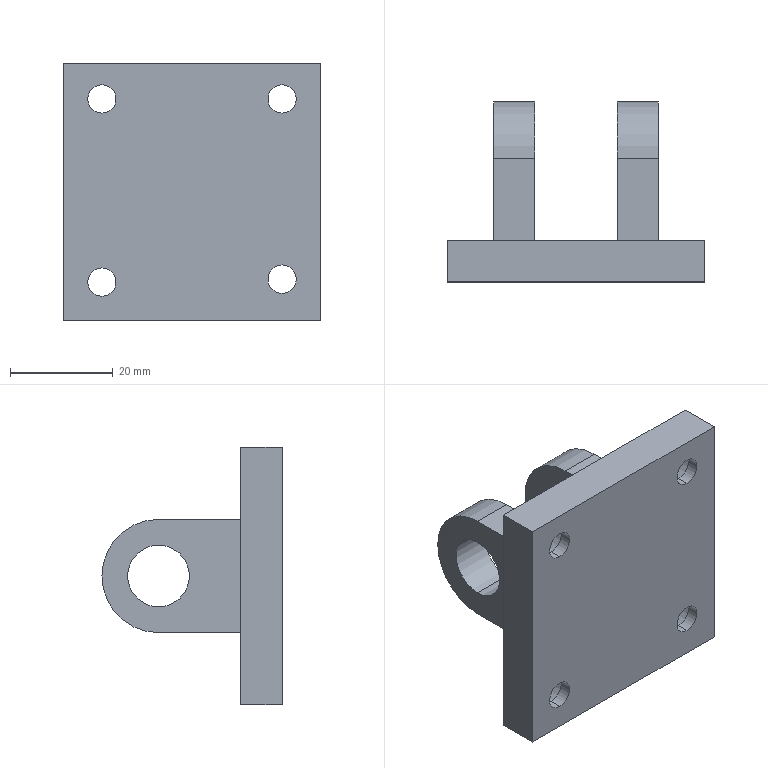Part | STEP file | X77-03301 | 1 solid | 42 faces | box 50 x 35 x 50 mm | volume 24854 mm3 | cylinder 24 | plane 18 | commonest cylinder face diameters 5.5 x8 10 x8 12 x4 22 x4
STEP:
#1=CARTESIAN_POINT('',(-1969.202,2.3,2.5));
#2=VERTEX_POINT('',#1);
#3=CARTESIAN_POINT('',(-1969.202,2.3,12.5));
#4=VERTEX_POINT('',#3);
#5=CARTESIAN_POINT('',(-1969.202,2.3,7.5));
#6=DIRECTION('',(0.,1.,0.));
#7=DIRECTION('',(0.,0.,1.));
#8=AXIS2_PLACEMENT_3D('',#5,#6,#7);
#9=CIRCLE('',#8,5.);
#10=EDGE_CURVE('',#2,#4,#9,.T.);
#11=ORIENTED_EDGE('',*,*,#10,.F.);
#12=CARTESIAN_POINT('',(-1969.202,8.,2.5));
#13=VERTEX_POINT('',#12);
#14=CARTESIAN_POINT('',(-1969.202,8.,2.5));
#15=DIRECTION('',(0.,1.,0.));
#16=VECTOR('',#15,1000.);
#17=LINE('',#14,#16);
#18=EDGE_CURVE('',#2,#13,#17,.T.);
#19=ORIENTED_EDGE('',*,*,#18,.T.);
#20=CARTESIAN_POINT('',(-1969.202,8.,12.5));
#21=VERTEX_POINT('',#20);
#22=CARTESIAN_POINT('',(-1969.202,8.,7.5));
#23=DIRECTION('',(0.,1.,0.));
#24=DIRECTION('',(0.,0.,1.));
#25=AXIS2_PLACEMENT_3D('',#22,#23,#24);
#26=CIRCLE('',#25,5.);
#27=EDGE_CURVE('',#13,#21,#26,.T.);
#28=ORIENTED_EDGE('',*,*,#27,.T.);
#29=CARTESIAN_POINT('',(-1969.202,8.,12.5));
#30=DIRECTION('',(0.,1.,0.));
#31=VECTOR('',#30,1000.);
#32=LINE('',#29,#31);
#33=EDGE_CURVE('',#4,#21,#32,.T.);
#34=ORIENTED_EDGE('',*,*,#33,.F.);
#35=EDGE_LOOP('',(#11,#19,#28,#34));
#36=FACE_OUTER_BOUND('',#35,.T.);
#37=CARTESIAN_POINT('',(-1969.202,8.,7.5));
#38=DIRECTION('',(0.,1.,0.));
#39=DIRECTION('',(0.,0.,1.));
#40=AXIS2_PLACEMENT_3D('',#37,#38,#39);
#41=CYLINDRICAL_SURFACE('',#40,5.);
#42=ADVANCED_FACE('',(#36),#41,.F.);
#43=CARTESIAN_POINT('',(-1969.202,0.,4.75));
#44=VERTEX_POINT('',#43);
#45=CARTESIAN_POINT('',(-1969.202,0.,10.25));
#46=VERTEX_POINT('',#45);
#47=CARTESIAN_POINT('',(-1969.202,0.,7.5));
#48=DIRECTION('',(0.,1.,0.));
#49=DIRECTION('',(0.,0.,1.));
#50=AXIS2_PLACEMENT_3D('',#47,#48,#49);
#51=CIRCLE('',#50,2.75);
#52=EDGE_CURVE('',#44,#46,#51,.T.);
#53=ORIENTED_EDGE('',*,*,#52,.F.);
#54=CARTESIAN_POINT('',(-1969.202,2.3,4.75));
#55=VERTEX_POINT('',#54);
#56=CARTESIAN_POINT('',(-1969.202,8.,4.75));
#57=DIRECTION('',(0.,1.,0.));
#58=VECTOR('',#57,1000.);
#59=LINE('',#56,#58);
#60=EDGE_CURVE('',#44,#55,#59,.T.);
#61=ORIENTED_EDGE('',*,*,#60,.T.);
#62=CARTESIAN_POINT('',(-1969.202,2.3,10.25));
#63=VERTEX_POINT('',#62);
#64=CARTESIAN_POINT('',(-1969.202,2.3,7.5));
#65=DIRECTION('',(0.,1.,0.));
#66=DIRECTION('',(0.,0.,1.));
#67=AXIS2_PLACEMENT_3D('',#64,#65,#66);
#68=CIRCLE('',#67,2.75);
#69=EDGE_CURVE('',#55,#63,#68,.T.);
#70=ORIENTED_EDGE('',*,*,#69,.T.);
#71=CARTESIAN_POINT('',(-1969.202,8.,10.25));
#72=DIRECTION('',(0.,1.,0.));
#73=VECTOR('',#72,1000.);
#74=LINE('',#71,#73);
#75=EDGE_CURVE('',#46,#63,#74,.T.);
#76=ORIENTED_EDGE('',*,*,#75,.F.);
#77=EDGE_LOOP('',(#53,#61,#70,#76));
#78=FACE_OUTER_BOUND('',#77,.T.);
#79=CARTESIAN_POINT('',(-1969.202,8.,7.5));
#80=DIRECTION('',(0.,1.,0.));
#81=DIRECTION('',(0.,0.,1.));
#82=AXIS2_PLACEMENT_3D('',#79,#80,#81);
#83=CYLINDRICAL_SURFACE('',#82,2.75);
#84=ADVANCED_FACE('',(#78),#83,.F.);
#85=CARTESIAN_POINT('',(-1934.202,2.3,3.072));
#86=VERTEX_POINT('',#85);
#87=CARTESIAN_POINT('',(-1934.202,2.3,13.072));
#88=VERTEX_POINT('',#87);
#89=CARTESIAN_POINT('',(-1934.202,2.3,8.072));
#90=DIRECTION('',(0.,1.,0.));
#91=DIRECTION('',(0.,0.,1.));
#92=AXIS2_PLACEMENT_3D('',#89,#90,#91);
#93=CIRCLE('',#92,5.);
#94=EDGE_CURVE('',#86,#88,#93,.T.);
#95=ORIENTED_EDGE('',*,*,#94,.F.);
#96=CARTESIAN_POINT('',(-1934.202,8.,3.072));
#97=VERTEX_POINT('',#96);
#98=CARTESIAN_POINT('',(-1934.202,8.,3.072));
#99=DIRECTION('',(0.,1.,0.));
#100=VECTOR('',#99,1000.);
#101=LINE('',#98,#100);
#102=EDGE_CURVE('',#86,#97,#101,.T.);
#103=ORIENTED_EDGE('',*,*,#102,.T.);
#104=CARTESIAN_POINT('',(-1934.202,8.,13.072));
#105=VERTEX_POINT('',#104);
#106=CARTESIAN_POINT('',(-1934.202,8.,8.072));
#107=DIRECTION('',(0.,1.,0.));
#108=DIRECTION('',(0.,0.,1.));
#109=AXIS2_PLACEMENT_3D('',#106,#107,#108);
#110=CIRCLE('',#109,5.);
#111=EDGE_CURVE('',#97,#105,#110,.T.);
#112=ORIENTED_EDGE('',*,*,#111,.T.);
#113=CARTESIAN_POINT('',(-1934.202,8.,13.072));
#114=DIRECTION('',(0.,1.,0.));
#115=VECTOR('',#114,1000.);
#116=LINE('',#113,#115);
#117=EDGE_CURVE('',#88,#105,#116,.T.);
#118=ORIENTED_EDGE('',*,*,#117,.F.);
#119=EDGE_LOOP('',(#95,#103,#112,#118));
#120=FACE_OUTER_BOUND('',#119,.T.);
#121=CARTESIAN_POINT('',(-1934.202,8.,8.072));
#122=DIRECTION('',(0.,1.,0.));
#123=DIRECTION('',(0.,0.,1.));
#124=AXIS2_PLACEMENT_3D('',#121,#122,#123);
#125=CYLINDRICAL_SURFACE('',#124,5.);
#126=ADVANCED_FACE('',(#120),#125,.F.);
#127=CARTESIAN_POINT('',(-1934.202,0.,5.322));
#128=VERTEX_POINT('',#127);
#129=CARTESIAN_POINT('',(-1934.202,0.,10.822));
#130=VERTEX_POINT('',#129);
#131=CARTESIAN_POINT('',(-1934.202,0.,8.072));
#132=DIRECTION('',(0.,1.,0.));
#133=DIRECTION('',(0.,0.,1.));
#134=AXIS2_PLACEMENT_3D('',#131,#132,#133);
#135=CIRCLE('',#134,2.75);
#136=EDGE_CURVE('',#128,#130,#135,.T.);
#137=ORIENTED_EDGE('',*,*,#136,.F.);
#138=CARTESIAN_POINT('',(-1934.202,2.3,5.322));
#139=VERTEX_POINT('',#138);
#140=CARTESIAN_POINT('',(-1934.202,8.,5.322));
#141=DIRECTION('',(0.,1.,0.));
#142=VECTOR('',#141,1000.);
#143=LINE('',#140,#142);
#144=EDGE_CURVE('',#128,#139,#143,.T.);
#145=ORIENTED_EDGE('',*,*,#144,.T.);
#146=CARTESIAN_POINT('',(-1934.202,2.3,10.822));
#147=VERTEX_POINT('',#146);
#148=CARTESIAN_POINT('',(-1934.202,2.3,8.072));
#149=DIRECTION('',(0.,1.,0.));
#150=DIRECTION('',(0.,0.,1.));
#151=AXIS2_PLACEMENT_3D('',#148,#149,#150);
#152=CIRCLE('',#151,2.75);
#153=EDGE_CURVE('',#139,#147,#152,.T.);
#154=ORIENTED_EDGE('',*,*,#153,.T.);
#155=CARTESIAN_POINT('',(-1934.202,8.,10.822));
#156=DIRECTION('',(0.,1.,0.));
#157=VECTOR('',#156,1000.);
#158=LINE('',#155,#157);
#159=EDGE_CURVE('',#130,#147,#158,.T.);
#160=ORIENTED_EDGE('',*,*,#159,.F.);
#161=EDGE_LOOP('',(#137,#145,#154,#160));
#162=FACE_OUTER_BOUND('',#161,.T.);
#163=CARTESIAN_POINT('',(-1934.202,8.,8.072));
#164=DIRECTION('',(0.,1.,0.));
#165=DIRECTION('',(0.,0.,1.));
#166=AXIS2_PLACEMENT_3D('',#163,#164,#165);
#167=CYLINDRICAL_SURFACE('',#166,2.75);
#168=ADVANCED_FACE('',(#162),#167,.F.);
#169=CARTESIAN_POINT('',(-1934.202,2.3,38.072));
#170=VERTEX_POINT('',#169);
#171=CARTESIAN_POINT('',(-1934.202,2.3,48.072));
#172=VERTEX_POINT('',#171);
#173=CARTESIAN_POINT('',(-1934.202,2.3,43.072));
#174=DIRECTION('',(0.,1.,0.));
#175=DIRECTION('',(0.,0.,1.));
#176=AXIS2_PLACEMENT_3D('',#173,#174,#175);
#177=CIRCLE('',#176,5.);
#178=EDGE_CURVE('',#170,#172,#177,.T.);
#179=ORIENTED_EDGE('',*,*,#178,.F.);
#180=CARTESIAN_POINT('',(-1934.202,8.,38.072));
#181=VERTEX_POINT('',#180);
#182=CARTESIAN_POINT('',(-1934.202,8.,38.072));
#183=DIRECTION('',(0.,1.,0.));
#184=VECTOR('',#183,1000.);
#185=LINE('',#182,#184);
#186=EDGE_CURVE('',#170,#181,#185,.T.);
#187=ORIENTED_EDGE('',*,*,#186,.T.);
#188=CARTESIAN_POINT('',(-1934.202,8.,48.072));
#189=VERTEX_POINT('',#188);
#190=CARTESIAN_POINT('',(-1934.202,8.,43.072));
#191=DIRECTION('',(0.,1.,0.));
#192=DIRECTION('',(0.,0.,1.));
#193=AXIS2_PLACEMENT_3D('',#190,#191,#192);
#194=CIRCLE('',#193,5.);
#195=EDGE_CURVE('',#181,#189,#194,.T.);
#196=ORIENTED_EDGE('',*,*,#195,.T.);
#197=CARTESIAN_POINT('',(-1934.202,8.,48.072));
#198=DIRECTION('',(0.,1.,0.));
#199=VECTOR('',#198,1000.);
#200=LINE('',#197,#199);
#201=EDGE_CURVE('',#172,#189,#200,.T.);
#202=ORIENTED_EDGE('',*,*,#201,.F.);
#203=EDGE_LOOP('',(#179,#187,#196,#202));
#204=FACE_OUTER_BOUND('',#203,.T.);
#205=CARTESIAN_POINT('',(-1934.202,8.,43.072));
#206=DIRECTION('',(0.,1.,0.));
#207=DIRECTION('',(0.,0.,1.));
#208=AXIS2_PLACEMENT_3D('',#205,#206,#207);
#209=CYLINDRICAL_SURFACE('',#208,5.);
#210=ADVANCED_FACE('',(#204),#209,.F.);
#211=CARTESIAN_POINT('',(-1934.202,0.,40.322));
#212=VERTEX_POINT('',#211);
#213=CARTESIAN_POINT('',(-1934.202,0.,45.822));
#214=VERTEX_POINT('',#213);
#215=CARTESIAN_POINT('',(-1934.202,0.,43.072));
#216=DIRECTION('',(0.,1.,0.));
#217=DIRECTION('',(0.,0.,1.));
#218=AXIS2_PLACEMENT_3D('',#215,#216,#217);
#219=CIRCLE('',#218,2.75);
#220=EDGE_CURVE('',#212,#214,#219,.T.);
#221=ORIENTED_EDGE('',*,*,#220,.F.);
#222=CARTESIAN_POINT('',(-1934.202,2.3,40.322));
#223=VERTEX_POINT('',#222);
#224=CARTESIAN_POINT('',(-1934.202,8.,40.322));
#225=DIRECTION('',(0.,1.,0.));
#226=VECTOR('',#225,1000.);
#227=LINE('',#224,#226);
#228=EDGE_CURVE('',#212,#223,#227,.T.);
#229=ORIENTED_EDGE('',*,*,#228,.T.);
#230=CARTESIAN_POINT('',(-1934.202,2.3,45.822));
#231=VERTEX_POINT('',#230);
#232=CARTESIAN_POINT('',(-1934.202,2.3,43.072));
#233=DIRECTION('',(0.,1.,0.));
#234=DIRECTION('',(0.,0.,1.));
#235=AXIS2_PLACEMENT_3D('',#232,#233,#234);
#236=CIRCLE('',#235,2.75);
#237=EDGE_CURVE('',#223,#231,#236,.T.);
#238=ORIENTED_EDGE('',*,*,#237,.T.);
#239=CARTESIAN_POINT('',(-1934.202,8.,45.822));
#240=DIRECTION('',(0.,1.,0.));
#241=VECTOR('',#240,1000.);
#242=LINE('',#239,#241);
#243=EDGE_CURVE('',#214,#231,#242,.T.);
#244=ORIENTED_EDGE('',*,*,#243,.F.);
#245=EDGE_LOOP('',(#221,#229,#238,#244));
#246=FACE_OUTER_BOUND('',#245,.T.);
#247=CARTESIAN_POINT('',(-1934.202,8.,43.072));
#248=DIRECTION('',(0.,1.,0.));
#249=DIRECTION('',(0.,0.,1.));
#250=AXIS2_PLACEMENT_3D('',#247,#248,#249);
#251=CYLINDRICAL_SURFACE('',#250,2.75);
#252=ADVANCED_FACE('',(#246),#251,.F.);
#253=CARTESIAN_POINT('',(-1969.202,2.3,38.072));
#254=VERTEX_POINT('',#253);
#255=CARTESIAN_POINT('',(-1969.202,2.3,48.072));
#256=VERTEX_POINT('',#255);
#257=CARTESIAN_POINT('',(-1969.202,2.3,43.072));
#258=DIRECTION('',(0.,1.,0.));
#259=DIRECTION('',(0.,0.,1.));
#260=AXIS2_PLACEMENT_3D('',#257,#258,#259);
#261=CIRCLE('',#260,5.);
#262=EDGE_CURVE('',#254,#256,#261,.T.);
#263=ORIENTED_EDGE('',*,*,#262,.F.);
#264=CARTESIAN_POINT('',(-1969.202,8.,38.072));
#265=VERTEX_POINT('',#264);
#266=CARTESIAN_POINT('',(-1969.202,8.,38.072));
#267=DIRECTION('',(0.,1.,0.));
#268=VECTOR('',#267,1000.);
#269=LINE('',#266,#268);
#270=EDGE_CURVE('',#254,#265,#269,.T.);
#271=ORIENTED_EDGE('',*,*,#270,.T.);
#272=CARTESIAN_POINT('',(-1969.202,8.,48.072));
#273=VERTEX_POINT('',#272);
#274=CARTESIAN_POINT('',(-1969.202,8.,43.072));
#275=DIRECTION('',(0.,1.,0.));
#276=DIRECTION('',(0.,0.,1.));
#277=AXIS2_PLACEMENT_3D('',#274,#275,#276);
#278=CIRCLE('',#277,5.);
#279=EDGE_CURVE('',#265,#273,#278,.T.);
#280=ORIENTED_EDGE('',*,*,#279,.T.);
#281=CARTESIAN_POINT('',(-1969.202,8.,48.072));
#282=DIRECTION('',(0.,1.,0.));
#283=VECTOR('',#282,1000.);
#284=LINE('',#281,#283);
#285=EDGE_CURVE('',#256,#273,#284,.T.);
#286=ORIENTED_EDGE('',*,*,#285,.F.);
#287=EDGE_LOOP('',(#263,#271,#280,#286));
#288=FACE_OUTER_BOUND('',#287,.T.);
#289=CARTESIAN_POINT('',(-1969.202,8.,43.072));
#290=DIRECTION('',(0.,1.,0.));
#291=DIRECTION('',(0.,0.,1.));
#292=AXIS2_PLACEMENT_3D('',#289,#290,#291);
#293=CYLINDRICAL_SURFACE('',#292,5.);
#294=ADVANCED_FACE('',(#288),#293,.F.);
#295=CARTESIAN_POINT('',(-1969.202,0.,40.322));
#296=VERTEX_POINT('',#295);
#297=CARTESIAN_POINT('',(-1969.202,0.,45.822));
#298=VERTEX_POINT('',#297);
#299=CARTESIAN_POINT('',(-1969.202,0.,43.072));
#300=DIRECTION('',(0.,1.,0.));
#301=DIRECTION('',(0.,0.,1.));
#302=AXIS2_PLACEMENT_3D('',#299,#300,#301);
#303=CIRCLE('',#302,2.75);
#304=EDGE_CURVE('',#296,#298,#303,.T.);
#305=ORIENTED_EDGE('',*,*,#304,.F.);
#306=CARTESIAN_POINT('',(-1969.202,2.3,40.322));
#307=VERTEX_POINT('',#306);
#308=CARTESIAN_POINT('',(-1969.202,8.,40.322));
#309=DIRECTION('',(0.,1.,0.));
#310=VECTOR('',#309,1000.);
#311=LINE('',#308,#310);
#312=EDGE_CURVE('',#296,#307,#311,.T.);
#313=ORIENTED_EDGE('',*,*,#312,.T.);
#314=CARTESIAN_POINT('',(-1969.202,2.3,45.822));
#315=VERTEX_POINT('',#314);
#316=CARTESIAN_POINT('',(-1969.202,2.3,43.072));
#317=DIRECTION('',(0.,1.,0.));
#318=DIRECTION('',(0.,0.,1.));
#319=AXIS2_PLACEMENT_3D('',#316,#317,#318);
#320=CIRCLE('',#319,2.75);
#321=EDGE_CURVE('',#307,#315,#320,.T.);
#322=ORIENTED_EDGE('',*,*,#321,.T.);
#323=CARTESIAN_POINT('',(-1969.202,8.,45.822));
#324=DIRECTION('',(0.,1.,0.));
#325=VECTOR('',#324,1000.);
#326=LINE('',#323,#325);
#327=EDGE_CURVE('',#298,#315,#326,.T.);
#328=ORIENTED_EDGE('',*,*,#327,.F.);
#329=EDGE_LOOP('',(#305,#313,#322,#328));
#330=FACE_OUTER_BOUND('',#329,.T.);
#331=CARTESIAN_POINT('',(-1969.202,8.,43.072));
#332=DIRECTION('',(0.,1.,0.));
#333=DIRECTION('',(0.,0.,1.));
#334=AXIS2_PLACEMENT_3D('',#331,#332,#333);
#335=CYLINDRICAL_SURFACE('',#334,2.75);
#336=ADVANCED_FACE('',(#330),#335,.F.);
#337=CARTESIAN_POINT('',(-1943.702,24.,31.));
#338=VERTEX_POINT('',#337);
#339=CARTESIAN_POINT('',(-1943.702,24.,19.));
#340=VERTEX_POINT('',#339);
#341=CARTESIAN_POINT('',(-1943.702,24.,25.));
#342=DIRECTION('',(1.,0.,0.));
#343=DIRECTION('',(0.,0.,-1.));
#344=AXIS2_PLACEMENT_3D('',#341,#342,#343);
#345=CIRCLE('',#344,6.);
#346=EDGE_CURVE('',#338,#340,#345,.T.);
#347=ORIENTED_EDGE('',*,*,#346,.F.);
#348=CARTESIAN_POINT('',(-1935.702,24.,31.));
#349=VERTEX_POINT('',#348);
#350=CARTESIAN_POINT('',(-1976.702,24.,31.));
#351=DIRECTION('',(1.,0.,0.));
#352=VECTOR('',#351,1000.);
#353=LINE('',#350,#352);
#354=EDGE_CURVE('',#338,#349,#353,.T.);
#355=ORIENTED_EDGE('',*,*,#354,.T.);
#356=CARTESIAN_POINT('',(-1935.702,24.,19.));
#357=VERTEX_POINT('',#356);
#358=CARTESIAN_POINT('',(-1935.702,24.,25.));
#359=DIRECTION('',(1.,0.,0.));
#360=DIRECTION('',(0.,0.,-1.));
#361=AXIS2_PLACEMENT_3D('',#358,#359,#360);
#362=CIRCLE('',#361,6.);
#363=EDGE_CURVE('',#349,#357,#362,.T.);
#364=ORIENTED_EDGE('',*,*,#363,.T.);
#365=CARTESIAN_POINT('',(-1976.702,24.,19.));
#366=DIRECTION('',(1.,0.,0.));
#367=VECTOR('',#366,1000.);
#368=LINE('',#365,#367);
#369=EDGE_CURVE('',#340,#357,#368,.T.);
#370=ORIENTED_EDGE('',*,*,#369,.F.);
#371=EDGE_LOOP('',(#347,#355,#364,#370));
#372=FACE_OUTER_BOUND('',#371,.T.);
#373=CARTESIAN_POINT('',(-1976.702,24.,25.));
#374=DIRECTION('',(1.,0.,0.));
#375=DIRECTION('',(0.,0.,-1.));
#376=AXIS2_PLACEMENT_3D('',#373,#374,#375);
#377=CYLINDRICAL_SURFACE('',#376,6.);
#378=ADVANCED_FACE('',(#372),#377,.F.);
#379=CARTESIAN_POINT('',(-1967.702,24.,31.));
#380=VERTEX_POINT('',#379);
#381=CARTESIAN_POINT('',(-1967.702,24.,19.));
#382=VERTEX_POINT('',#381);
#383=CARTESIAN_POINT('',(-1967.702,24.,25.));
#384=DIRECTION('',(1.,0.,0.));
#385=DIRECTION('',(0.,0.,-1.));
#386=AXIS2_PLACEMENT_3D('',#383,#384,#385);
#387=CIRCLE('',#386,6.);
#388=EDGE_CURVE('',#380,#382,#387,.T.);
#389=ORIENTED_EDGE('',*,*,#388,.F.);
#390=CARTESIAN_POINT('',(-1959.702,24.,31.));
#391=VERTEX_POINT('',#390);
#392=CARTESIAN_POINT('',(-1976.702,24.,31.));
#393=DIRECTION('',(1.,0.,0.));
#394=VECTOR('',#393,1000.);
#395=LINE('',#392,#394);
#396=EDGE_CURVE('',#380,#391,#395,.T.);
#397=ORIENTED_EDGE('',*,*,#396,.T.);
#398=CARTESIAN_POINT('',(-1959.702,24.,19.));
#399=VERTEX_POINT('',#398);
#400=CARTESIAN_POINT('',(-1959.702,24.,25.));
#401=DIRECTION('',(-1.,0.,0.));
#402=DIRECTION('',(0.,0.,1.));
#403=AXIS2_PLACEMENT_3D('',#400,#401,#402);
#404=CIRCLE('',#403,6.);
#405=EDGE_CURVE('',#399,#391,#404,.T.);
#406=ORIENTED_EDGE('',*,*,#405,.F.);
#407=CARTESIAN_POINT('',(-1976.702,24.,19.));
#408=DIRECTION('',(1.,0.,0.));
#409=VECTOR('',#408,1000.);
#410=LINE('',#407,#409);
#411=EDGE_CURVE('',#382,#399,#410,.T.);
#412=ORIENTED_EDGE('',*,*,#411,.F.);
#413=EDGE_LOOP('',(#389,#397,#406,#412));
#414=FACE_OUTER_BOUND('',#413,.T.);
#415=CARTESIAN_POINT('',(-1976.702,24.,25.));
#416=DIRECTION('',(1.,0.,0.));
#417=DIRECTION('',(0.,0.,-1.));
#418=AXIS2_PLACEMENT_3D('',#415,#416,#417);
#419=CYLINDRICAL_SURFACE('',#418,6.);
#420=ADVANCED_FACE('',(#414),#419,.F.);
#421=CARTESIAN_POINT('',(-1967.702,24.,25.));
#422=DIRECTION('',(1.,0.,0.));
#423=DIRECTION('',(0.,0.,-1.));
#424=AXIS2_PLACEMENT_3D('',#421,#422,#423);
#425=CIRCLE('',#424,6.);
#426=EDGE_CURVE('',#382,#380,#425,.T.);
#427=ORIENTED_EDGE('',*,*,#426,.T.);
#428=ORIENTED_EDGE('',*,*,#388,.T.);
#429=EDGE_LOOP('',(#427,#428));
#430=FACE_BOUND('',#429,.T.);
#431=CARTESIAN_POINT('',(-1967.702,24.,36.));
#432=VERTEX_POINT('',#431);
#433=CARTESIAN_POINT('',(-1967.702,35.,25.));
#434=VERTEX_POINT('',#433);
#435=CARTESIAN_POINT('',(-1967.702,24.,25.));
#436=DIRECTION('',(-1.,0.,0.));
#437=DIRECTION('',(0.,0.,-1.));
#438=AXIS2_PLACEMENT_3D('',#435,#436,#437);
#439=CIRCLE('',#438,11.);
#440=EDGE_CURVE('',#432,#434,#439,.T.);
#441=ORIENTED_EDGE('',*,*,#440,.T.);
#442=CARTESIAN_POINT('',(-1967.702,24.,14.));
#443=VERTEX_POINT('',#442);
#444=CARTESIAN_POINT('',(-1967.702,24.,25.));
#445=DIRECTION('',(-1.,0.,0.));
#446=DIRECTION('',(0.,0.,-1.));
#447=AXIS2_PLACEMENT_3D('',#444,#445,#446);
#448=CIRCLE('',#447,11.);
#449=EDGE_CURVE('',#434,#443,#448,.T.);
#450=ORIENTED_EDGE('',*,*,#449,.T.);
#451=CARTESIAN_POINT('',(-1967.702,8.,14.));
#452=VERTEX_POINT('',#451);
#453=CARTESIAN_POINT('',(-1967.702,8.,14.));
#454=DIRECTION('',(0.,1.,0.));
#455=VECTOR('',#454,1000.);
#456=LINE('',#453,#455);
#457=EDGE_CURVE('',#452,#443,#456,.T.);
#458=ORIENTED_EDGE('',*,*,#457,.F.);
#459=CARTESIAN_POINT('',(-1967.702,8.,36.));
#460=VERTEX_POINT('',#459);
#461=CARTESIAN_POINT('',(-1967.702,8.,50.));
#462=DIRECTION('',(0.,0.,-1.));
#463=VECTOR('',#462,1000.);
#464=LINE('',#461,#463);
#465=EDGE_CURVE('',#460,#452,#464,.T.);
#466=ORIENTED_EDGE('',*,*,#465,.F.);
#467=CARTESIAN_POINT('',(-1967.702,8.,36.));
#468=DIRECTION('',(0.,-1.,0.));
#469=VECTOR('',#468,1000.);
#470=LINE('',#467,#469);
#471=EDGE_CURVE('',#432,#460,#470,.T.);
#472=ORIENTED_EDGE('',*,*,#471,.F.);
#473=EDGE_LOOP('',(#441,#450,#458,#466,#472));
#474=FACE_OUTER_BOUND('',#473,.T.);
#475=CARTESIAN_POINT('',(-1967.702,8.,50.));
#476=DIRECTION('',(1.,0.,0.));
#477=DIRECTION('',(0.,0.,-1.));
#478=AXIS2_PLACEMENT_3D('',#475,#476,#477);
#479=PLANE('',#478);
#480=ADVANCED_FACE('',(#430,#474),#479,.F.);
#481=CARTESIAN_POINT('',(-1935.702,24.,25.));
#482=DIRECTION('',(1.,0.,0.));
#483=DIRECTION('',(0.,0.,-1.));
#484=AXIS2_PLACEMENT_3D('',#481,#482,#483);
#485=CIRCLE('',#484,6.);
#486=EDGE_CURVE('',#357,#349,#485,.T.);
#487=ORIENTED_EDGE('',*,*,#486,.F.);
#488=ORIENTED_EDGE('',*,*,#363,.F.);
#489=EDGE_LOOP('',(#487,#488));
#490=FACE_BOUND('',#489,.T.);
#491=CARTESIAN_POINT('',(-1935.702,8.,14.));
#492=VERTEX_POINT('',#491);
#493=CARTESIAN_POINT('',(-1935.702,24.,14.));
#494=VERTEX_POINT('',#493);
#495=CARTESIAN_POINT('',(-1935.702,21.5,14.));
#496=DIRECTION('',(0.,1.,0.));
#497=VECTOR('',#496,1000.);
#498=LINE('',#495,#497);
#499=EDGE_CURVE('',#492,#494,#498,.T.);
#500=ORIENTED_EDGE('',*,*,#499,.T.);
#501=CARTESIAN_POINT('',(-1935.702,35.,25.));
#502=VERTEX_POINT('',#501);
#503=CARTESIAN_POINT('',(-1935.702,24.,25.));
#504=DIRECTION('',(1.,0.,0.));
#505=DIRECTION('',(0.,0.,1.));
#506=AXIS2_PLACEMENT_3D('',#503,#504,#505);
#507=CIRCLE('',#506,11.);
#508=EDGE_CURVE('',#494,#502,#507,.T.);
#509=ORIENTED_EDGE('',*,*,#508,.T.);
#510=CARTESIAN_POINT('',(-1935.702,24.,36.));
#511=VERTEX_POINT('',#510);
#512=CARTESIAN_POINT('',(-1935.702,24.,25.));
#513=DIRECTION('',(1.,0.,0.));
#514=DIRECTION('',(0.,0.,1.));
#515=AXIS2_PLACEMENT_3D('',#512,#513,#514);
#516=CIRCLE('',#515,11.);
#517=EDGE_CURVE('',#502,#511,#516,.T.);
#518=ORIENTED_EDGE('',*,*,#517,.T.);
#519=CARTESIAN_POINT('',(-1935.702,8.,36.));
#520=VERTEX_POINT('',#519);
#521=CARTESIAN_POINT('',(-1935.702,21.5,36.));
#522=DIRECTION('',(0.,-1.,0.));
#523=VECTOR('',#522,1000.);
#524=LINE('',#521,#523);
#525=EDGE_CURVE('',#511,#520,#524,.T.);
#526=ORIENTED_EDGE('',*,*,#525,.T.);
#527=CARTESIAN_POINT('',(-1935.702,8.,50.));
#528=DIRECTION('',(0.,0.,-1.));
#529=VECTOR('',#528,1000.);
#530=LINE('',#527,#529);
#531=EDGE_CURVE('',#520,#492,#530,.T.);
#532=ORIENTED_EDGE('',*,*,#531,.T.);
#533=EDGE_LOOP('',(#500,#509,#518,#526,#532));
#534=FACE_OUTER_BOUND('',#533,.T.);
#535=CARTESIAN_POINT('',(-1935.702,35.,50.));
#536=DIRECTION('',(-1.,0.,0.));
#537=DIRECTION('',(0.,0.,1.));
#538=AXIS2_PLACEMENT_3D('',#535,#536,#537);
#539=PLANE('',#538);
#540=ADVANCED_FACE('',(#490,#534),#539,.F.);
#541=CARTESIAN_POINT('',(-1943.702,24.,25.));
#542=DIRECTION('',(1.,0.,0.));
#543=DIRECTION('',(0.,0.,-1.));
#544=AXIS2_PLACEMENT_3D('',#541,#542,#543);
#545=CIRCLE('',#544,6.);
#546=EDGE_CURVE('',#340,#338,#545,.T.);
#547=ORIENTED_EDGE('',*,*,#546,.T.);
#548=ORIENTED_EDGE('',*,*,#346,.T.);
#549=EDGE_LOOP('',(#547,#548));
#550=FACE_BOUND('',#549,.T.);
#551=CARTESIAN_POINT('',(-1943.702,24.,36.));
#552=VERTEX_POINT('',#551);
#553=CARTESIAN_POINT('',(-1943.702,35.,25.));
#554=VERTEX_POINT('',#553);
#555=CARTESIAN_POINT('',(-1943.702,24.,25.));
#556=DIRECTION('',(-1.,0.,0.));
#557=DIRECTION('',(0.,0.,-1.));
#558=AXIS2_PLACEMENT_3D('',#555,#556,#557);
#559=CIRCLE('',#558,11.);
#560=EDGE_CURVE('',#552,#554,#559,.T.);
#561=ORIENTED_EDGE('',*,*,#560,.T.);
#562=CARTESIAN_POINT('',(-1943.702,24.,14.));
#563=VERTEX_POINT('',#562);
#564=CARTESIAN_POINT('',(-1943.702,24.,25.));
#565=DIRECTION('',(-1.,0.,0.));
#566=DIRECTION('',(0.,0.,-1.));
#567=AXIS2_PLACEMENT_3D('',#564,#565,#566);
#568=CIRCLE('',#567,11.);
#569=EDGE_CURVE('',#554,#563,#568,.T.);
#570=ORIENTED_EDGE('',*,*,#569,.T.);
#571=CARTESIAN_POINT('',(-1943.702,8.,14.));
#572=VERTEX_POINT('',#571);
#573=CARTESIAN_POINT('',(-1943.702,8.,14.));
#574=DIRECTION('',(0.,1.,0.));
#575=VECTOR('',#574,1000.);
#576=LINE('',#573,#575);
#577=EDGE_CURVE('',#572,#563,#576,.T.);
#578=ORIENTED_EDGE('',*,*,#577,.F.);
#579=CARTESIAN_POINT('',(-1943.702,8.,36.));
#580=VERTEX_POINT('',#579);
#581=CARTESIAN_POINT('',(-1943.702,8.,50.));
#582=DIRECTION('',(0.,0.,-1.));
#583=VECTOR('',#582,1000.);
#584=LINE('',#581,#583);
#585=EDGE_CURVE('',#580,#572,#584,.T.);
#586=ORIENTED_EDGE('',*,*,#585,.F.);
#587=CARTESIAN_POINT('',(-1943.702,8.,36.));
#588=DIRECTION('',(0.,-1.,0.));
#589=VECTOR('',#588,1000.);
#590=LINE('',#587,#589);
#591=EDGE_CURVE('',#552,#580,#590,.T.);
#592=ORIENTED_EDGE('',*,*,#591,.F.);
#593=EDGE_LOOP('',(#561,#570,#578,#586,#592));
#594=FACE_OUTER_BOUND('',#593,.T.);
#595=CARTESIAN_POINT('',(-1943.702,8.,50.));
#596=DIRECTION('',(1.,0.,0.));
#597=DIRECTION('',(0.,0.,-1.));
#598=AXIS2_PLACEMENT_3D('',#595,#596,#597);
#599=PLANE('',#598);
#600=ADVANCED_FACE('',(#550,#594),#599,.F.);
#601=ORIENTED_EDGE('',*,*,#405,.T.);
#602=CARTESIAN_POINT('',(-1959.702,24.,25.));
#603=DIRECTION('',(-1.,0.,0.));
#604=DIRECTION('',(0.,0.,1.));
#605=AXIS2_PLACEMENT_3D('',#602,#603,#604);
#606=CIRCLE('',#605,6.);
#607=EDGE_CURVE('',#391,#399,#606,.T.);
#608=ORIENTED_EDGE('',*,*,#607,.T.);
#609=EDGE_LOOP('',(#601,#608));
#610=FACE_BOUND('',#609,.T.);
#611=CARTESIAN_POINT('',(-1959.702,24.,14.));
#612=VERTEX_POINT('',#611);
#613=CARTESIAN_POINT('',(-1959.702,8.,14.));
#614=VERTEX_POINT('',#613);
#615=CARTESIAN_POINT('',(-1959.702,35.,14.));
#616=DIRECTION('',(0.,-1.,0.));
#617=VECTOR('',#616,1000.);
#618=LINE('',#615,#617);
#619=EDGE_CURVE('',#612,#614,#618,.T.);
#620=ORIENTED_EDGE('',*,*,#619,.F.);
#621=CARTESIAN_POINT('',(-1959.702,35.,25.));
#622=VERTEX_POINT('',#621);
#623=CARTESIAN_POINT('',(-1959.702,24.,25.));
#624=DIRECTION('',(1.,0.,0.));
#625=DIRECTION('',(0.,0.,1.));
#626=AXIS2_PLACEMENT_3D('',#623,#624,#625);
#627=CIRCLE('',#626,11.);
#628=EDGE_CURVE('',#612,#622,#627,.T.);
#629=ORIENTED_EDGE('',*,*,#628,.T.);
#630=CARTESIAN_POINT('',(-1959.702,24.,36.));
#631=VERTEX_POINT('',#630);
#632=CARTESIAN_POINT('',(-1959.702,24.,25.));
#633=DIRECTION('',(1.,0.,0.));
#634=DIRECTION('',(0.,0.,1.));
#635=AXIS2_PLACEMENT_3D('',#632,#633,#634);
#636=CIRCLE('',#635,11.);
#637=EDGE_CURVE('',#622,#631,#636,.T.);
#638=ORIENTED_EDGE('',*,*,#637,.T.);
#639=CARTESIAN_POINT('',(-1959.702,8.,36.));
#640=VERTEX_POINT('',#639);
#641=CARTESIAN_POINT('',(-1959.702,35.,36.));
#642=DIRECTION('',(0.,1.,0.));
#643=VECTOR('',#642,1000.);
#644=LINE('',#641,#643);
#645=EDGE_CURVE('',#640,#631,#644,.T.);
#646=ORIENTED_EDGE('',*,*,#645,.F.);
#647=CARTESIAN_POINT('',(-1959.702,8.,50.));
#648=DIRECTION('',(0.,0.,-1.));
#649=VECTOR('',#648,1000.);
#650=LINE('',#647,#649);
#651=EDGE_CURVE('',#640,#614,#650,.T.);
#652=ORIENTED_EDGE('',*,*,#651,.T.);
#653=EDGE_LOOP('',(#620,#629,#638,#646,#652));
#654=FACE_OUTER_BOUND('',#653,.T.);
#655=CARTESIAN_POINT('',(-1959.702,35.,50.));
#656=DIRECTION('',(-1.,0.,0.));
#657=DIRECTION('',(0.,0.,1.));
#658=AXIS2_PLACEMENT_3D('',#655,#656,#657);
#659=PLANE('',#658);
#660=ADVANCED_FACE('',(#610,#654),#659,.F.);
#661=CARTESIAN_POINT('',(-1976.702,8.,0.));
#662=VERTEX_POINT('',#661);
#663=CARTESIAN_POINT('',(-1976.702,0.,0.));
#664=VERTEX_POINT('',#663);
#665=CARTESIAN_POINT('',(-1976.702,0.,0.));
#666=DIRECTION('',(0.,-1.,0.));
#667=VECTOR('',#666,1000.);
#668=LINE('',#665,#667);
#669=EDGE_CURVE('',#662,#664,#668,.T.);
#670=ORIENTED_EDGE('',*,*,#669,.T.);
#671=CARTESIAN_POINT('',(-1976.702,0.,50.));
#672=VERTEX_POINT('',#671);
#673=CARTESIAN_POINT('',(-1976.702,0.,50.));
#674=DIRECTION('',(0.,0.,-1.));
#675=VECTOR('',#674,1000.);
#676=LINE('',#673,#675);
#677=EDGE_CURVE('',#672,#664,#676,.T.);
#678=ORIENTED_EDGE('',*,*,#677,.F.);
#679=CARTESIAN_POINT('',(-1976.702,8.,50.));
#680=VERTEX_POINT('',#679);
#681=CARTESIAN_POINT('',(-1976.702,0.,50.));
#682=DIRECTION('',(0.,-1.,0.));
#683=VECTOR('',#682,1000.);
#684=LINE('',#681,#683);
#685=EDGE_CURVE('',#680,#672,#684,.T.);
#686=ORIENTED_EDGE('',*,*,#685,.F.);
#687=CARTESIAN_POINT('',(-1976.702,8.,50.));
#688=DIRECTION('',(0.,0.,-1.));
#689=VECTOR('',#688,1000.);
#690=LINE('',#687,#689);
#691=EDGE_CURVE('',#680,#662,#690,.T.);
#692=ORIENTED_EDGE('',*,*,#691,.T.);
#693=EDGE_LOOP('',(#670,#678,#686,#692));
#694=FACE_OUTER_BOUND('',#693,.T.);
#695=CARTESIAN_POINT('',(-1976.702,0.,50.));
#696=DIRECTION('',(1.,0.,0.));
#697=DIRECTION('',(0.,0.,-1.));
#698=AXIS2_PLACEMENT_3D('',#695,#696,#697);
#699=PLANE('',#698);
#700=ADVANCED_FACE('',(#694),#699,.F.);
#701=CARTESIAN_POINT('',(-1969.202,0.,7.5));
#702=DIRECTION('',(0.,1.,0.));
#703=DIRECTION('',(0.,0.,1.));
#704=AXIS2_PLACEMENT_3D('',#701,#702,#703);
#705=CIRCLE('',#704,2.75);
#706=EDGE_CURVE('',#46,#44,#705,.T.);
#707=ORIENTED_EDGE('',*,*,#706,.T.);
#708=ORIENTED_EDGE('',*,*,#52,.T.);
#709=EDGE_LOOP('',(#707,#708));
#710=FACE_BOUND('',#709,.T.);
#711=CARTESIAN_POINT('',(-1934.202,0.,8.072));
#712=DIRECTION('',(0.,1.,0.));
#713=DIRECTION('',(0.,0.,1.));
#714=AXIS2_PLACEMENT_3D('',#711,#712,#713);
#715=CIRCLE('',#714,2.75);
#716=EDGE_CURVE('',#130,#128,#715,.T.);
#717=ORIENTED_EDGE('',*,*,#716,.T.);
#718=ORIENTED_EDGE('',*,*,#136,.T.);
#719=EDGE_LOOP('',(#717,#718));
#720=FACE_BOUND('',#719,.T.);
#721=CARTESIAN_POINT('',(-1934.202,0.,43.072));
#722=DIRECTION('',(0.,1.,0.));
#723=DIRECTION('',(0.,0.,1.));
#724=AXIS2_PLACEMENT_3D('',#721,#722,#723);
#725=CIRCLE('',#724,2.75);
#726=EDGE_CURVE('',#214,#212,#725,.T.);
#727=ORIENTED_EDGE('',*,*,#726,.T.);
#728=ORIENTED_EDGE('',*,*,#220,.T.);
#729=EDGE_LOOP('',(#727,#728));
#730=FACE_BOUND('',#729,.T.);
#731=CARTESIAN_POINT('',(-1969.202,0.,43.072));
#732=DIRECTION('',(0.,1.,0.));
#733=DIRECTION('',(0.,0.,1.));
#734=AXIS2_PLACEMENT_3D('',#731,#732,#733);
#735=CIRCLE('',#734,2.75);
#736=EDGE_CURVE('',#298,#296,#735,.T.);
#737=ORIENTED_EDGE('',*,*,#736,.T.);
#738=ORIENTED_EDGE('',*,*,#304,.T.);
#739=EDGE_LOOP('',(#737,#738));
#740=FACE_BOUND('',#739,.T.);
#741=CARTESIAN_POINT('',(-1926.702,0.,0.));
#742=VERTEX_POINT('',#741);
#743=CARTESIAN_POINT('',(-1926.702,0.,0.));
#744=DIRECTION('',(1.,0.,0.));
#745=VECTOR('',#744,1000.);
#746=LINE('',#743,#745);
#747=EDGE_CURVE('',#664,#742,#746,.T.);
#748=ORIENTED_EDGE('',*,*,#747,.T.);
#749=CARTESIAN_POINT('',(-1926.702,0.,50.));
#750=VERTEX_POINT('',#749);
#751=CARTESIAN_POINT('',(-1926.702,0.,50.));
#752=DIRECTION('',(0.,0.,-1.));
#753=VECTOR('',#752,1000.);
#754=LINE('',#751,#753);
#755=EDGE_CURVE('',#750,#742,#754,.T.);
#756=ORIENTED_EDGE('',*,*,#755,.F.);
#757=CARTESIAN_POINT('',(-1926.702,0.,50.));
#758=DIRECTION('',(1.,0.,0.));
#759=VECTOR('',#758,1000.);
#760=LINE('',#757,#759);
#761=EDGE_CURVE('',#672,#750,#760,.T.);
#762=ORIENTED_EDGE('',*,*,#761,.F.);
#763=ORIENTED_EDGE('',*,*,#677,.T.);
#764=EDGE_LOOP('',(#748,#756,#762,#763));
#765=FACE_OUTER_BOUND('',#764,.T.);
#766=CARTESIAN_POINT('',(-1926.702,0.,50.));
#767=DIRECTION('',(0.,1.,0.));
#768=DIRECTION('',(-1.,0.,0.));
#769=AXIS2_PLACEMENT_3D('',#766,#767,#768);
#770=PLANE('',#769);
#771=ADVANCED_FACE('',(#710,#720,#730,#740,#765),#770,.F.);
#772=CARTESIAN_POINT('',(-1926.702,8.,0.));
#773=VERTEX_POINT('',#772);
#774=CARTESIAN_POINT('',(-1926.702,8.,0.));
#775=DIRECTION('',(0.,1.,0.));
#776=VECTOR('',#775,1000.);
#777=LINE('',#774,#776);
#778=EDGE_CURVE('',#742,#773,#777,.T.);
#779=ORIENTED_EDGE('',*,*,#778,.T.);
#780=CARTESIAN_POINT('',(-1926.702,8.,50.));
#781=VERTEX_POINT('',#780);
#782=CARTESIAN_POINT('',(-1926.702,8.,50.));
#783=DIRECTION('',(0.,0.,-1.));
#784=VECTOR('',#783,1000.);
#785=LINE('',#782,#784);
#786=EDGE_CURVE('',#781,#773,#785,.T.);
#787=ORIENTED_EDGE('',*,*,#786,.F.);
#788=CARTESIAN_POINT('',(-1926.702,8.,50.));
#789=DIRECTION('',(0.,1.,0.));
#790=VECTOR('',#789,1000.);
#791=LINE('',#788,#790);
#792=EDGE_CURVE('',#750,#781,#791,.T.);
#793=ORIENTED_EDGE('',*,*,#792,.F.);
#794=ORIENTED_EDGE('',*,*,#755,.T.);
#795=EDGE_LOOP('',(#779,#787,#793,#794));
#796=FACE_OUTER_BOUND('',#795,.T.);
#797=CARTESIAN_POINT('',(-1926.702,8.,50.));
#798=DIRECTION('',(-1.,0.,0.));
#799=DIRECTION('',(0.,0.,1.));
#800=AXIS2_PLACEMENT_3D('',#797,#798,#799);
#801=PLANE('',#800);
#802=ADVANCED_FACE('',(#796),#801,.F.);
#803=CARTESIAN_POINT('',(-1969.202,8.,7.5));
#804=DIRECTION('',(0.,1.,0.));
#805=DIRECTION('',(0.,0.,1.));
#806=AXIS2_PLACEMENT_3D('',#803,#804,#805);
#807=CIRCLE('',#806,5.);
#808=EDGE_CURVE('',#21,#13,#807,.T.);
#809=ORIENTED_EDGE('',*,*,#808,.F.);
#810=ORIENTED_EDGE('',*,*,#27,.F.);
#811=EDGE_LOOP('',(#809,#810));
#812=FACE_BOUND('',#811,.T.);
#813=CARTESIAN_POINT('',(-1934.202,8.,8.072));
#814=DIRECTION('',(0.,1.,0.));
#815=DIRECTION('',(0.,0.,1.));
#816=AXIS2_PLACEMENT_3D('',#813,#814,#815);
#817=CIRCLE('',#816,5.);
#818=EDGE_CURVE('',#105,#97,#817,.T.);
#819=ORIENTED_EDGE('',*,*,#818,.F.);
#820=ORIENTED_EDGE('',*,*,#111,.F.);
#821=EDGE_LOOP('',(#819,#820));
#822=FACE_BOUND('',#821,.T.);
#823=CARTESIAN_POINT('',(-1934.202,8.,43.072));
#824=DIRECTION('',(0.,1.,0.));
#825=DIRECTION('',(0.,0.,1.));
#826=AXIS2_PLACEMENT_3D('',#823,#824,#825);
#827=CIRCLE('',#826,5.);
#828=EDGE_CURVE('',#189,#181,#827,.T.);
#829=ORIENTED_EDGE('',*,*,#828,.F.);
#830=ORIENTED_EDGE('',*,*,#195,.F.);
#831=EDGE_LOOP('',(#829,#830));
#832=FACE_BOUND('',#831,.T.);
#833=CARTESIAN_POINT('',(-1969.202,8.,43.072));
#834=DIRECTION('',(0.,1.,0.));
#835=DIRECTION('',(0.,0.,1.));
#836=AXIS2_PLACEMENT_3D('',#833,#834,#835);
#837=CIRCLE('',#836,5.);
#838=EDGE_CURVE('',#273,#265,#837,.T.);
#839=ORIENTED_EDGE('',*,*,#838,.F.);
#840=ORIENTED_EDGE('',*,*,#279,.F.);
#841=EDGE_LOOP('',(#839,#840));
#842=FACE_BOUND('',#841,.T.);
#843=CARTESIAN_POINT('',(-1959.702,8.,0.));
#844=DIRECTION('',(-1.,0.,0.));
#845=VECTOR('',#844,1000.);
#846=LINE('',#843,#845);
#847=EDGE_CURVE('',#773,#662,#846,.T.);
#848=ORIENTED_EDGE('',*,*,#847,.T.);
#849=ORIENTED_EDGE('',*,*,#691,.F.);
#850=CARTESIAN_POINT('',(-1976.702,8.,50.));
#851=DIRECTION('',(-1.,0.,0.));
#852=VECTOR('',#851,1000.);
#853=LINE('',#850,#852);
#854=EDGE_CURVE('',#781,#680,#853,.T.);
#855=ORIENTED_EDGE('',*,*,#854,.F.);
#856=ORIENTED_EDGE('',*,*,#786,.T.);
#857=EDGE_LOOP('',(#848,#849,#855,#856));
#858=FACE_OUTER_BOUND('',#857,.T.);
#859=ORIENTED_EDGE('',*,*,#465,.T.);
#860=CARTESIAN_POINT('',(-1976.702,8.,14.));
#861=DIRECTION('',(1.,0.,0.));
#862=VECTOR('',#861,1000.);
#863=LINE('',#860,#862);
#864=EDGE_CURVE('',#452,#614,#863,.T.);
#865=ORIENTED_EDGE('',*,*,#864,.T.);
#866=ORIENTED_EDGE('',*,*,#651,.F.);
#867=CARTESIAN_POINT('',(-1976.702,8.,36.));
#868=DIRECTION('',(1.,0.,0.));
#869=VECTOR('',#868,1000.);
#870=LINE('',#867,#869);
#871=EDGE_CURVE('',#460,#640,#870,.T.);
#872=ORIENTED_EDGE('',*,*,#871,.F.);
#873=EDGE_LOOP('',(#859,#865,#866,#872));
#874=FACE_BOUND('',#873,.T.);
#875=ORIENTED_EDGE('',*,*,#585,.T.);
#876=CARTESIAN_POINT('',(-1976.702,8.,14.));
#877=DIRECTION('',(1.,0.,0.));
#878=VECTOR('',#877,1000.);
#879=LINE('',#876,#878);
#880=EDGE_CURVE('',#572,#492,#879,.T.);
#881=ORIENTED_EDGE('',*,*,#880,.T.);
#882=ORIENTED_EDGE('',*,*,#531,.F.);
#883=CARTESIAN_POINT('',(-1976.702,8.,36.));
#884=DIRECTION('',(1.,0.,0.));
#885=VECTOR('',#884,1000.);
#886=LINE('',#883,#885);
#887=EDGE_CURVE('',#580,#520,#886,.T.);
#888=ORIENTED_EDGE('',*,*,#887,.F.);
#889=EDGE_LOOP('',(#875,#881,#882,#888));
#890=FACE_BOUND('',#889,.T.);
#891=CARTESIAN_POINT('',(-1959.702,8.,50.));
#892=DIRECTION('',(0.,-1.,0.));
#893=DIRECTION('',(0.,0.,-1.));
#894=AXIS2_PLACEMENT_3D('',#891,#892,#893);
#895=PLANE('',#894);
#896=ADVANCED_FACE('',(#812,#822,#832,#842,#858,#874,#890),#895,.F.);
#897=ORIENTED_EDGE('',*,*,#792,.T.);
#898=ORIENTED_EDGE('',*,*,#854,.T.);
#899=ORIENTED_EDGE('',*,*,#685,.T.);
#900=ORIENTED_EDGE('',*,*,#761,.T.);
#901=EDGE_LOOP('',(#897,#898,#899,#900));
#902=FACE_OUTER_BOUND('',#901,.T.);
#903=CARTESIAN_POINT('',(-1959.702,35.,50.));
#904=DIRECTION('',(0.,0.,-1.));
#905=DIRECTION('',(-1.,0.,0.));
#906=AXIS2_PLACEMENT_3D('',#903,#904,#905);
#907=PLANE('',#906);
#908=ADVANCED_FACE('',(#902),#907,.F.);
#909=ORIENTED_EDGE('',*,*,#847,.F.);
#910=ORIENTED_EDGE('',*,*,#778,.F.);
#911=ORIENTED_EDGE('',*,*,#747,.F.);
#912=ORIENTED_EDGE('',*,*,#669,.F.);
#913=EDGE_LOOP('',(#909,#910,#911,#912));
#914=FACE_OUTER_BOUND('',#913,.T.);
#915=CARTESIAN_POINT('',(-1959.702,35.,0.));
#916=DIRECTION('',(0.,0.,-1.));
#917=DIRECTION('',(-1.,0.,0.));
#918=AXIS2_PLACEMENT_3D('',#915,#916,#917);
#919=PLANE('',#918);
#920=ADVANCED_FACE('',(#914),#919,.T.);
#921=ORIENTED_EDGE('',*,*,#645,.T.);
#922=CARTESIAN_POINT('',(-1967.702,24.,36.));
#923=DIRECTION('',(-1.,0.,0.));
#924=VECTOR('',#923,1000.);
#925=LINE('',#922,#924);
#926=EDGE_CURVE('',#631,#432,#925,.T.);
#927=ORIENTED_EDGE('',*,*,#926,.T.);
#928=ORIENTED_EDGE('',*,*,#471,.T.);
#929=ORIENTED_EDGE('',*,*,#871,.T.);
#930=EDGE_LOOP('',(#921,#927,#928,#929));
#931=FACE_OUTER_BOUND('',#930,.T.);
#932=CARTESIAN_POINT('',(-1976.702,21.5,36.));
#933=DIRECTION('',(0.,0.,1.));
#934=DIRECTION('',(1.,0.,0.));
#935=AXIS2_PLACEMENT_3D('',#932,#933,#934);
#936=PLANE('',#935);
#937=ADVANCED_FACE('',(#931),#936,.T.);
#938=ORIENTED_EDGE('',*,*,#525,.F.);
#939=CARTESIAN_POINT('',(-1943.702,24.,36.));
#940=DIRECTION('',(-1.,0.,0.));
#941=VECTOR('',#940,1000.);
#942=LINE('',#939,#941);
#943=EDGE_CURVE('',#511,#552,#942,.T.);
#944=ORIENTED_EDGE('',*,*,#943,.T.);
#945=ORIENTED_EDGE('',*,*,#591,.T.);
#946=ORIENTED_EDGE('',*,*,#887,.T.);
#947=EDGE_LOOP('',(#938,#944,#945,#946));
#948=FACE_OUTER_BOUND('',#947,.T.);
#949=CARTESIAN_POINT('',(-1976.702,21.5,36.));
#950=DIRECTION('',(0.,0.,1.));
#951=DIRECTION('',(1.,0.,0.));
#952=AXIS2_PLACEMENT_3D('',#949,#950,#951);
#953=PLANE('',#952);
#954=ADVANCED_FACE('',(#948),#953,.T.);
#955=ORIENTED_EDGE('',*,*,#457,.T.);
#956=CARTESIAN_POINT('',(-1959.702,24.,14.));
#957=DIRECTION('',(1.,0.,0.));
#958=VECTOR('',#957,1000.);
#959=LINE('',#956,#958);
#960=EDGE_CURVE('',#443,#612,#959,.T.);
#961=ORIENTED_EDGE('',*,*,#960,.T.);
#962=ORIENTED_EDGE('',*,*,#619,.T.);
#963=ORIENTED_EDGE('',*,*,#864,.F.);
#964=EDGE_LOOP('',(#955,#961,#962,#963));
#965=FACE_OUTER_BOUND('',#964,.T.);
#966=CARTESIAN_POINT('',(-1976.702,21.5,14.));
#967=DIRECTION('',(0.,0.,-1.));
#968=DIRECTION('',(-1.,0.,0.));
#969=AXIS2_PLACEMENT_3D('',#966,#967,#968);
#970=PLANE('',#969);
#971=ADVANCED_FACE('',(#965),#970,.T.);
#972=ORIENTED_EDGE('',*,*,#577,.T.);
#973=CARTESIAN_POINT('',(-1935.702,24.,14.));
#974=DIRECTION('',(1.,0.,0.));
#975=VECTOR('',#974,1000.);
#976=LINE('',#973,#975);
#977=EDGE_CURVE('',#563,#494,#976,.T.);
#978=ORIENTED_EDGE('',*,*,#977,.T.);
#979=ORIENTED_EDGE('',*,*,#499,.F.);
#980=ORIENTED_EDGE('',*,*,#880,.F.);
#981=EDGE_LOOP('',(#972,#978,#979,#980));
#982=FACE_OUTER_BOUND('',#981,.T.);
#983=CARTESIAN_POINT('',(-1976.702,21.5,14.));
#984=DIRECTION('',(0.,0.,-1.));
#985=DIRECTION('',(-1.,0.,0.));
#986=AXIS2_PLACEMENT_3D('',#983,#984,#985);
#987=PLANE('',#986);
#988=ADVANCED_FACE('',(#982),#987,.T.);
#989=ORIENTED_EDGE('',*,*,#396,.F.);
#990=ORIENTED_EDGE('',*,*,#426,.F.);
#991=ORIENTED_EDGE('',*,*,#411,.T.);
#992=ORIENTED_EDGE('',*,*,#607,.F.);
#993=EDGE_LOOP('',(#989,#990,#991,#992));
#994=FACE_OUTER_BOUND('',#993,.T.);
#995=CARTESIAN_POINT('',(-1976.702,24.,25.));
#996=DIRECTION('',(1.,0.,0.));
#997=DIRECTION('',(0.,0.,-1.));
#998=AXIS2_PLACEMENT_3D('',#995,#996,#997);
#999=CYLINDRICAL_SURFACE('',#998,6.);
#1000=ADVANCED_FACE('',(#994),#999,.F.);
#1001=ORIENTED_EDGE('',*,*,#354,.F.);
#1002=ORIENTED_EDGE('',*,*,#546,.F.);
#1003=ORIENTED_EDGE('',*,*,#369,.T.);
#1004=ORIENTED_EDGE('',*,*,#486,.T.);
#1005=EDGE_LOOP('',(#1001,#1002,#1003,#1004));
#1006=FACE_OUTER_BOUND('',#1005,.T.);
#1007=CARTESIAN_POINT('',(-1976.702,24.,25.));
#1008=DIRECTION('',(1.,0.,0.));
#1009=DIRECTION('',(0.,0.,-1.));
#1010=AXIS2_PLACEMENT_3D('',#1007,#1008,#1009);
#1011=CYLINDRICAL_SURFACE('',#1010,6.);
#1012=ADVANCED_FACE('',(#1006),#1011,.F.);
#1013=CARTESIAN_POINT('',(-1935.702,35.,25.));
#1014=DIRECTION('',(1.,0.,0.));
#1015=VECTOR('',#1014,1000.);
#1016=LINE('',#1013,#1015);
#1017=EDGE_CURVE('',#554,#502,#1016,.T.);
#1018=ORIENTED_EDGE('',*,*,#1017,.F.);
#1019=ORIENTED_EDGE('',*,*,#560,.F.);
#1020=ORIENTED_EDGE('',*,*,#943,.F.);
#1021=ORIENTED_EDGE('',*,*,#517,.F.);
#1022=EDGE_LOOP('',(#1018,#1019,#1020,#1021));
#1023=FACE_OUTER_BOUND('',#1022,.T.);
#1024=CARTESIAN_POINT('',(-1943.702,24.,25.));
#1025=DIRECTION('',(-1.,0.,0.));
#1026=DIRECTION('',(0.,0.,1.));
#1027=AXIS2_PLACEMENT_3D('',#1024,#1025,#1026);
#1028=CYLINDRICAL_SURFACE('',#1027,11.);
#1029=ADVANCED_FACE('',(#1023),#1028,.T.);
#1030=ORIENTED_EDGE('',*,*,#569,.F.);
#1031=ORIENTED_EDGE('',*,*,#1017,.T.);
#1032=ORIENTED_EDGE('',*,*,#508,.F.);
#1033=ORIENTED_EDGE('',*,*,#977,.F.);
#1034=EDGE_LOOP('',(#1030,#1031,#1032,#1033));
#1035=FACE_OUTER_BOUND('',#1034,.T.);
#1036=CARTESIAN_POINT('',(-1976.702,24.,25.));
#1037=DIRECTION('',(-1.,0.,0.));
#1038=DIRECTION('',(0.,0.,1.));
#1039=AXIS2_PLACEMENT_3D('',#1036,#1037,#1038);
#1040=CYLINDRICAL_SURFACE('',#1039,11.);
#1041=ADVANCED_FACE('',(#1035),#1040,.T.);
#1042=CARTESIAN_POINT('',(-1959.702,35.,25.));
#1043=DIRECTION('',(1.,0.,0.));
#1044=VECTOR('',#1043,1000.);
#1045=LINE('',#1042,#1044);
#1046=EDGE_CURVE('',#434,#622,#1045,.T.);
#1047=ORIENTED_EDGE('',*,*,#1046,.F.);
#1048=ORIENTED_EDGE('',*,*,#440,.F.);
#1049=ORIENTED_EDGE('',*,*,#926,.F.);
#1050=ORIENTED_EDGE('',*,*,#637,.F.);
#1051=EDGE_LOOP('',(#1047,#1048,#1049,#1050));
#1052=FACE_OUTER_BOUND('',#1051,.T.);
#1053=CARTESIAN_POINT('',(-1967.702,24.,25.));
#1054=DIRECTION('',(-1.,0.,0.));
#1055=DIRECTION('',(0.,0.,1.));
#1056=AXIS2_PLACEMENT_3D('',#1053,#1054,#1055);
#1057=CYLINDRICAL_SURFACE('',#1056,11.);
#1058=ADVANCED_FACE('',(#1052),#1057,.T.);
#1059=ORIENTED_EDGE('',*,*,#449,.F.);
#1060=ORIENTED_EDGE('',*,*,#1046,.T.);
#1061=ORIENTED_EDGE('',*,*,#628,.F.);
#1062=ORIENTED_EDGE('',*,*,#960,.F.);
#1063=EDGE_LOOP('',(#1059,#1060,#1061,#1062));
#1064=FACE_OUTER_BOUND('',#1063,.T.);
#1065=CARTESIAN_POINT('',(-1976.702,24.,25.));
#1066=DIRECTION('',(-1.,0.,0.));
#1067=DIRECTION('',(0.,0.,1.));
#1068=AXIS2_PLACEMENT_3D('',#1065,#1066,#1067);
#1069=CYLINDRICAL_SURFACE('',#1068,11.);
#1070=ADVANCED_FACE('',(#1064),#1069,.T.);
#1071=ORIENTED_EDGE('',*,*,#312,.F.);
#1072=ORIENTED_EDGE('',*,*,#736,.F.);
#1073=ORIENTED_EDGE('',*,*,#327,.T.);
#1074=CARTESIAN_POINT('',(-1969.202,2.3,43.072));
#1075=DIRECTION('',(0.,1.,0.));
#1076=DIRECTION('',(0.,0.,1.));
#1077=AXIS2_PLACEMENT_3D('',#1074,#1075,#1076);
#1078=CIRCLE('',#1077,2.75);
#1079=EDGE_CURVE('',#315,#307,#1078,.T.);
#1080=ORIENTED_EDGE('',*,*,#1079,.T.);
#1081=EDGE_LOOP('',(#1071,#1072,#1073,#1080));
#1082=FACE_OUTER_BOUND('',#1081,.T.);
#1083=CARTESIAN_POINT('',(-1969.202,8.,43.072));
#1084=DIRECTION('',(0.,1.,0.));
#1085=DIRECTION('',(0.,0.,1.));
#1086=AXIS2_PLACEMENT_3D('',#1083,#1084,#1085);
#1087=CYLINDRICAL_SURFACE('',#1086,2.75);
#1088=ADVANCED_FACE('',(#1082),#1087,.F.);
#1089=ORIENTED_EDGE('',*,*,#1079,.F.);
#1090=ORIENTED_EDGE('',*,*,#321,.F.);
#1091=EDGE_LOOP('',(#1089,#1090));
#1092=FACE_BOUND('',#1091,.T.);
#1093=CARTESIAN_POINT('',(-1969.202,2.3,43.072));
#1094=DIRECTION('',(0.,1.,0.));
#1095=DIRECTION('',(0.,0.,1.));
#1096=AXIS2_PLACEMENT_3D('',#1093,#1094,#1095);
#1097=CIRCLE('',#1096,5.);
#1098=EDGE_CURVE('',#256,#254,#1097,.T.);
#1099=ORIENTED_EDGE('',*,*,#1098,.T.);
#1100=ORIENTED_EDGE('',*,*,#262,.T.);
#1101=EDGE_LOOP('',(#1099,#1100));
#1102=FACE_OUTER_BOUND('',#1101,.T.);
#1103=CARTESIAN_POINT('',(-1966.452,2.3,43.072));
#1104=DIRECTION('',(0.,-1.,0.));
#1105=DIRECTION('',(0.,0.,-1.));
#1106=AXIS2_PLACEMENT_3D('',#1103,#1104,#1105);
#1107=PLANE('',#1106);
#1108=ADVANCED_FACE('',(#1092,#1102),#1107,.F.);
#1109=ORIENTED_EDGE('',*,*,#270,.F.);
#1110=ORIENTED_EDGE('',*,*,#1098,.F.);
#1111=ORIENTED_EDGE('',*,*,#285,.T.);
#1112=ORIENTED_EDGE('',*,*,#838,.T.);
#1113=EDGE_LOOP('',(#1109,#1110,#1111,#1112));
#1114=FACE_OUTER_BOUND('',#1113,.T.);
#1115=CARTESIAN_POINT('',(-1969.202,8.,43.072));
#1116=DIRECTION('',(0.,1.,0.));
#1117=DIRECTION('',(0.,0.,1.));
#1118=AXIS2_PLACEMENT_3D('',#1115,#1116,#1117);
#1119=CYLINDRICAL_SURFACE('',#1118,5.);
#1120=ADVANCED_FACE('',(#1114),#1119,.F.);
#1121=ORIENTED_EDGE('',*,*,#228,.F.);
#1122=ORIENTED_EDGE('',*,*,#726,.F.);
#1123=ORIENTED_EDGE('',*,*,#243,.T.);
#1124=CARTESIAN_POINT('',(-1934.202,2.3,43.072));
#1125=DIRECTION('',(0.,1.,0.));
#1126=DIRECTION('',(0.,0.,1.));
#1127=AXIS2_PLACEMENT_3D('',#1124,#1125,#1126);
#1128=CIRCLE('',#1127,2.75);
#1129=EDGE_CURVE('',#231,#223,#1128,.T.);
#1130=ORIENTED_EDGE('',*,*,#1129,.T.);
#1131=EDGE_LOOP('',(#1121,#1122,#1123,#1130));
#1132=FACE_OUTER_BOUND('',#1131,.T.);
#1133=CARTESIAN_POINT('',(-1934.202,8.,43.072));
#1134=DIRECTION('',(0.,1.,0.));
#1135=DIRECTION('',(0.,0.,1.));
#1136=AXIS2_PLACEMENT_3D('',#1133,#1134,#1135);
#1137=CYLINDRICAL_SURFACE('',#1136,2.75);
#1138=ADVANCED_FACE('',(#1132),#1137,.F.);
#1139=ORIENTED_EDGE('',*,*,#1129,.F.);
#1140=ORIENTED_EDGE('',*,*,#237,.F.);
#1141=EDGE_LOOP('',(#1139,#1140));
#1142=FACE_BOUND('',#1141,.T.);
#1143=CARTESIAN_POINT('',(-1934.202,2.3,43.072));
#1144=DIRECTION('',(0.,1.,0.));
#1145=DIRECTION('',(0.,0.,1.));
#1146=AXIS2_PLACEMENT_3D('',#1143,#1144,#1145);
#1147=CIRCLE('',#1146,5.);
#1148=EDGE_CURVE('',#172,#170,#1147,.T.);
#1149=ORIENTED_EDGE('',*,*,#1148,.T.);
#1150=ORIENTED_EDGE('',*,*,#178,.T.);
#1151=EDGE_LOOP('',(#1149,#1150));
#1152=FACE_OUTER_BOUND('',#1151,.T.);
#1153=CARTESIAN_POINT('',(-1931.452,2.3,43.072));
#1154=DIRECTION('',(0.,-1.,0.));
#1155=DIRECTION('',(0.,0.,-1.));
#1156=AXIS2_PLACEMENT_3D('',#1153,#1154,#1155);
#1157=PLANE('',#1156);
#1158=ADVANCED_FACE('',(#1142,#1152),#1157,.F.);
#1159=ORIENTED_EDGE('',*,*,#186,.F.);
#1160=ORIENTED_EDGE('',*,*,#1148,.F.);
#1161=ORIENTED_EDGE('',*,*,#201,.T.);
#1162=ORIENTED_EDGE('',*,*,#828,.T.);
#1163=EDGE_LOOP('',(#1159,#1160,#1161,#1162));
#1164=FACE_OUTER_BOUND('',#1163,.T.);
#1165=CARTESIAN_POINT('',(-1934.202,8.,43.072));
#1166=DIRECTION('',(0.,1.,0.));
#1167=DIRECTION('',(0.,0.,1.));
#1168=AXIS2_PLACEMENT_3D('',#1165,#1166,#1167);
#1169=CYLINDRICAL_SURFACE('',#1168,5.);
#1170=ADVANCED_FACE('',(#1164),#1169,.F.);
#1171=ORIENTED_EDGE('',*,*,#144,.F.);
#1172=ORIENTED_EDGE('',*,*,#716,.F.);
#1173=ORIENTED_EDGE('',*,*,#159,.T.);
#1174=CARTESIAN_POINT('',(-1934.202,2.3,8.072));
#1175=DIRECTION('',(0.,1.,0.));
#1176=DIRECTION('',(0.,0.,1.));
#1177=AXIS2_PLACEMENT_3D('',#1174,#1175,#1176);
#1178=CIRCLE('',#1177,2.75);
#1179=EDGE_CURVE('',#147,#139,#1178,.T.);
#1180=ORIENTED_EDGE('',*,*,#1179,.T.);
#1181=EDGE_LOOP('',(#1171,#1172,#1173,#1180));
#1182=FACE_OUTER_BOUND('',#1181,.T.);
#1183=CARTESIAN_POINT('',(-1934.202,8.,8.072));
#1184=DIRECTION('',(0.,1.,0.));
#1185=DIRECTION('',(0.,0.,1.));
#1186=AXIS2_PLACEMENT_3D('',#1183,#1184,#1185);
#1187=CYLINDRICAL_SURFACE('',#1186,2.75);
#1188=ADVANCED_FACE('',(#1182),#1187,.F.);
#1189=ORIENTED_EDGE('',*,*,#1179,.F.);
#1190=ORIENTED_EDGE('',*,*,#153,.F.);
#1191=EDGE_LOOP('',(#1189,#1190));
#1192=FACE_BOUND('',#1191,.T.);
#1193=CARTESIAN_POINT('',(-1934.202,2.3,8.072));
#1194=DIRECTION('',(0.,1.,0.));
#1195=DIRECTION('',(0.,0.,1.));
#1196=AXIS2_PLACEMENT_3D('',#1193,#1194,#1195);
#1197=CIRCLE('',#1196,5.);
#1198=EDGE_CURVE('',#88,#86,#1197,.T.);
#1199=ORIENTED_EDGE('',*,*,#1198,.T.);
#1200=ORIENTED_EDGE('',*,*,#94,.T.);
#1201=EDGE_LOOP('',(#1199,#1200));
#1202=FACE_OUTER_BOUND('',#1201,.T.);
#1203=CARTESIAN_POINT('',(-1931.452,2.3,8.072));
#1204=DIRECTION('',(0.,-1.,0.));
#1205=DIRECTION('',(0.,0.,-1.));
#1206=AXIS2_PLACEMENT_3D('',#1203,#1204,#1205);
#1207=PLANE('',#1206);
#1208=ADVANCED_FACE('',(#1192,#1202),#1207,.F.);
#1209=ORIENTED_EDGE('',*,*,#102,.F.);
#1210=ORIENTED_EDGE('',*,*,#1198,.F.);
#1211=ORIENTED_EDGE('',*,*,#117,.T.);
#1212=ORIENTED_EDGE('',*,*,#818,.T.);
#1213=EDGE_LOOP('',(#1209,#1210,#1211,#1212));
#1214=FACE_OUTER_BOUND('',#1213,.T.);
#1215=CARTESIAN_POINT('',(-1934.202,8.,8.072));
#1216=DIRECTION('',(0.,1.,0.));
#1217=DIRECTION('',(0.,0.,1.));
#1218=AXIS2_PLACEMENT_3D('',#1215,#1216,#1217);
#1219=CYLINDRICAL_SURFACE('',#1218,5.);
#1220=ADVANCED_FACE('',(#1214),#1219,.F.);
#1221=ORIENTED_EDGE('',*,*,#60,.F.);
#1222=ORIENTED_EDGE('',*,*,#706,.F.);
#1223=ORIENTED_EDGE('',*,*,#75,.T.);
#1224=CARTESIAN_POINT('',(-1969.202,2.3,7.5));
#1225=DIRECTION('',(0.,1.,0.));
#1226=DIRECTION('',(0.,0.,1.));
#1227=AXIS2_PLACEMENT_3D('',#1224,#1225,#1226);
#1228=CIRCLE('',#1227,2.75);
#1229=EDGE_CURVE('',#63,#55,#1228,.T.);
#1230=ORIENTED_EDGE('',*,*,#1229,.T.);
#1231=EDGE_LOOP('',(#1221,#1222,#1223,#1230));
#1232=FACE_OUTER_BOUND('',#1231,.T.);
#1233=CARTESIAN_POINT('',(-1969.202,8.,7.5));
#1234=DIRECTION('',(0.,1.,0.));
#1235=DIRECTION('',(0.,0.,1.));
#1236=AXIS2_PLACEMENT_3D('',#1233,#1234,#1235);
#1237=CYLINDRICAL_SURFACE('',#1236,2.75);
#1238=ADVANCED_FACE('',(#1232),#1237,.F.);
#1239=ORIENTED_EDGE('',*,*,#1229,.F.);
#1240=ORIENTED_EDGE('',*,*,#69,.F.);
#1241=EDGE_LOOP('',(#1239,#1240));
#1242=FACE_BOUND('',#1241,.T.);
#1243=CARTESIAN_POINT('',(-1969.202,2.3,7.5));
#1244=DIRECTION('',(0.,1.,0.));
#1245=DIRECTION('',(0.,0.,1.));
#1246=AXIS2_PLACEMENT_3D('',#1243,#1244,#1245);
#1247=CIRCLE('',#1246,5.);
#1248=EDGE_CURVE('',#4,#2,#1247,.T.);
#1249=ORIENTED_EDGE('',*,*,#1248,.T.);
#1250=ORIENTED_EDGE('',*,*,#10,.T.);
#1251=EDGE_LOOP('',(#1249,#1250));
#1252=FACE_OUTER_BOUND('',#1251,.T.);
#1253=CARTESIAN_POINT('',(-1966.452,2.3,7.5));
#1254=DIRECTION('',(0.,-1.,0.));
#1255=DIRECTION('',(0.,0.,-1.));
#1256=AXIS2_PLACEMENT_3D('',#1253,#1254,#1255);
#1257=PLANE('',#1256);
#1258=ADVANCED_FACE('',(#1242,#1252),#1257,.F.);
#1259=ORIENTED_EDGE('',*,*,#18,.F.);
#1260=ORIENTED_EDGE('',*,*,#1248,.F.);
#1261=ORIENTED_EDGE('',*,*,#33,.T.);
#1262=ORIENTED_EDGE('',*,*,#808,.T.);
#1263=EDGE_LOOP('',(#1259,#1260,#1261,#1262));
#1264=FACE_OUTER_BOUND('',#1263,.T.);
#1265=CARTESIAN_POINT('',(-1969.202,8.,7.5));
#1266=DIRECTION('',(0.,1.,0.));
#1267=DIRECTION('',(0.,0.,1.));
#1268=AXIS2_PLACEMENT_3D('',#1265,#1266,#1267);
#1269=CYLINDRICAL_SURFACE('',#1268,5.);
#1270=ADVANCED_FACE('',(#1264),#1269,.F.);
#1271=CLOSED_SHELL('',(#42,#84,#126,#168,#210,#252,#294,#336,#378,#420,#480,#540,#600,#660,#700,#771,#802,#896,#908,#920,#937,#954,#971,#988,#1000,#1012,#1029,#1041,#1058,#1070,#1088,#1108,#1120,#1138,#1158,#1170,#1188,#1208,#1220,#1238,#1258,#1270));
#1272=MANIFOLD_SOLID_BREP('',#1271);
#1273=CARTESIAN_POINT('',(0.,0.,0.));
#1274=DIRECTION('',(0.,0.,1.));
#1275=DIRECTION('',(1.,0.,0.));
#1276=AXIS2_PLACEMENT_3D('',#1273,#1274,#1275);
#1277=(LENGTH_UNIT()NAMED_UNIT(*)SI_UNIT(.MILLI.,.METRE.));
#1278=UNCERTAINTY_MEASURE_WITH_UNIT(LENGTH_MEASURE(0.00001),#1277,'','');
#1279=(NAMED_UNIT(*)PLANE_ANGLE_UNIT()SI_UNIT($,.RADIAN.));
#1280=(NAMED_UNIT(*)SI_UNIT($,.STERADIAN.)SOLID_ANGLE_UNIT());
#1281=(GEOMETRIC_REPRESENTATION_CONTEXT(3)GLOBAL_UNCERTAINTY_ASSIGNED_CONTEXT((#1278))GLOBAL_UNIT_ASSIGNED_CONTEXT((#1277,#1279,#1280))REPRESENTATION_CONTEXT('',''));
#1282=ADVANCED_BREP_SHAPE_REPRESENTATION('',(#1272,#1276),#1281);